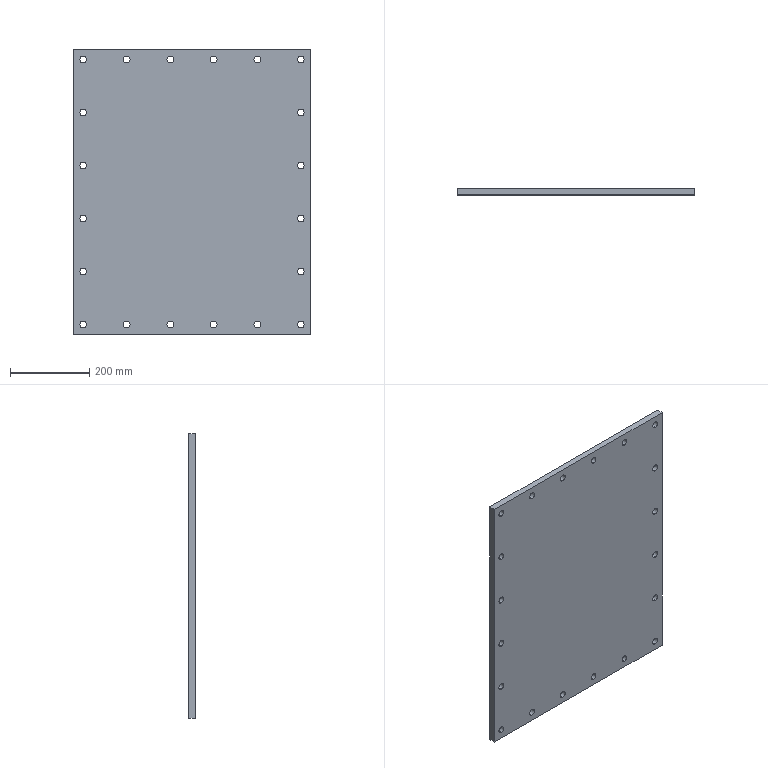Part | SolidWorks | features Extrusion 1, HoleWzd 1 | 1 solid | 46 faces | box 600 x 16 x 720 mm | volume 6839366 mm3 | cylinder 40 | plane 6 | commonest cylinder face diameters 17 x40